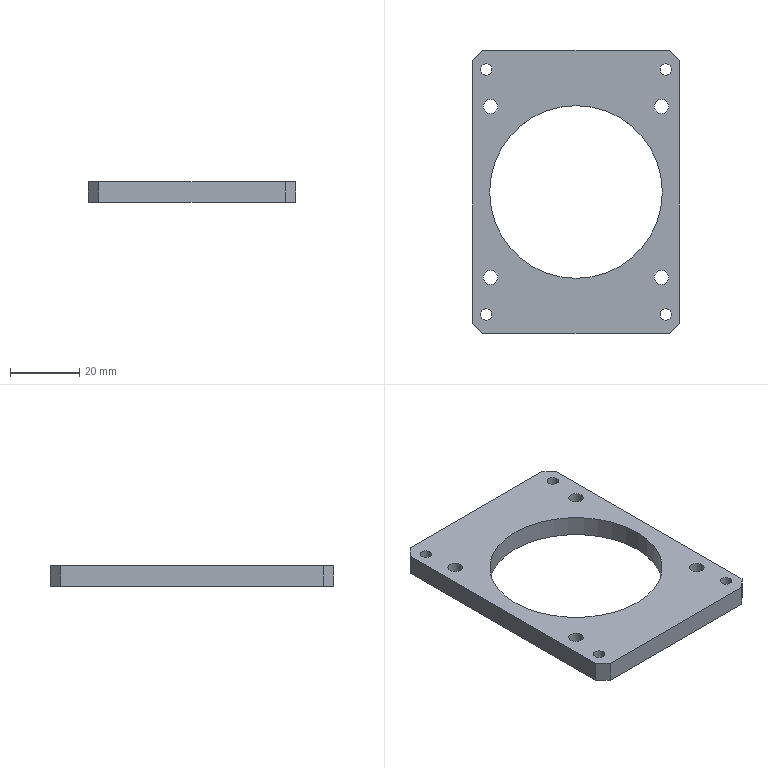Part | SolidWorks | features BaseBody 1 | 1 solid | 28 faces | box 60 x 82 x 6 mm | volume 17093 mm3 | cylinder 18 | plane 10 | commonest cylinder face diameters 3.3 x8 4.2 x8 50 x2
STEP:
#1=CARTESIAN_POINT('',(-24.35,35.5,6.));
#2=VERTEX_POINT('',#1);
#3=CARTESIAN_POINT('',(-27.65,35.5,6.));
#4=VERTEX_POINT('',#3);
#5=CARTESIAN_POINT('',(-26.,35.5,6.));
#6=DIRECTION('',(0.,0.,-1.));
#7=DIRECTION('',(-1.,0.,0.));
#8=AXIS2_PLACEMENT_3D('',#5,#6,#7);
#9=CIRCLE('',#8,1.65);
#10=EDGE_CURVE('',#2,#4,#9,.T.);
#11=ORIENTED_EDGE('',*,*,#10,.F.);
#12=CARTESIAN_POINT('',(-24.35,35.5,0.));
#13=VERTEX_POINT('',#12);
#14=CARTESIAN_POINT('',(-24.35,35.5,0.));
#15=DIRECTION('',(0.,0.,-1.));
#16=VECTOR('',#15,1000.);
#17=LINE('',#14,#16);
#18=EDGE_CURVE('',#2,#13,#17,.T.);
#19=ORIENTED_EDGE('',*,*,#18,.T.);
#20=CARTESIAN_POINT('',(-27.65,35.5,0.));
#21=VERTEX_POINT('',#20);
#22=CARTESIAN_POINT('',(-26.,35.5,0.));
#23=DIRECTION('',(0.,0.,1.));
#24=DIRECTION('',(-1.,0.,0.));
#25=AXIS2_PLACEMENT_3D('',#22,#23,#24);
#26=CIRCLE('',#25,1.65);
#27=EDGE_CURVE('',#21,#13,#26,.T.);
#28=ORIENTED_EDGE('',*,*,#27,.F.);
#29=CARTESIAN_POINT('',(-27.65,35.5,0.));
#30=DIRECTION('',(0.,0.,-1.));
#31=VECTOR('',#30,1000.);
#32=LINE('',#29,#31);
#33=EDGE_CURVE('',#4,#21,#32,.T.);
#34=ORIENTED_EDGE('',*,*,#33,.F.);
#35=EDGE_LOOP('',(#11,#19,#28,#34));
#36=FACE_OUTER_BOUND('',#35,.T.);
#37=CARTESIAN_POINT('',(-26.,35.5,0.));
#38=DIRECTION('',(0.,0.,-1.));
#39=DIRECTION('',(-1.,0.,0.));
#40=AXIS2_PLACEMENT_3D('',#37,#38,#39);
#41=CYLINDRICAL_SURFACE('',#40,1.65);
#42=ADVANCED_FACE('',(#36),#41,.F.);
#43=CARTESIAN_POINT('',(-24.35,-35.5,6.));
#44=VERTEX_POINT('',#43);
#45=CARTESIAN_POINT('',(-27.65,-35.5,6.));
#46=VERTEX_POINT('',#45);
#47=CARTESIAN_POINT('',(-26.,-35.5,6.));
#48=DIRECTION('',(0.,0.,-1.));
#49=DIRECTION('',(-1.,0.,0.));
#50=AXIS2_PLACEMENT_3D('',#47,#48,#49);
#51=CIRCLE('',#50,1.65);
#52=EDGE_CURVE('',#44,#46,#51,.T.);
#53=ORIENTED_EDGE('',*,*,#52,.F.);
#54=CARTESIAN_POINT('',(-24.35,-35.5,0.));
#55=VERTEX_POINT('',#54);
#56=CARTESIAN_POINT('',(-24.35,-35.5,0.));
#57=DIRECTION('',(0.,0.,-1.));
#58=VECTOR('',#57,1000.);
#59=LINE('',#56,#58);
#60=EDGE_CURVE('',#44,#55,#59,.T.);
#61=ORIENTED_EDGE('',*,*,#60,.T.);
#62=CARTESIAN_POINT('',(-27.65,-35.5,0.));
#63=VERTEX_POINT('',#62);
#64=CARTESIAN_POINT('',(-26.,-35.5,0.));
#65=DIRECTION('',(0.,0.,1.));
#66=DIRECTION('',(-1.,0.,0.));
#67=AXIS2_PLACEMENT_3D('',#64,#65,#66);
#68=CIRCLE('',#67,1.65);
#69=EDGE_CURVE('',#63,#55,#68,.T.);
#70=ORIENTED_EDGE('',*,*,#69,.F.);
#71=CARTESIAN_POINT('',(-27.65,-35.5,0.));
#72=DIRECTION('',(0.,0.,-1.));
#73=VECTOR('',#72,1000.);
#74=LINE('',#71,#73);
#75=EDGE_CURVE('',#46,#63,#74,.T.);
#76=ORIENTED_EDGE('',*,*,#75,.F.);
#77=EDGE_LOOP('',(#53,#61,#70,#76));
#78=FACE_OUTER_BOUND('',#77,.T.);
#79=CARTESIAN_POINT('',(-26.,-35.5,0.));
#80=DIRECTION('',(0.,0.,-1.));
#81=DIRECTION('',(-1.,0.,0.));
#82=AXIS2_PLACEMENT_3D('',#79,#80,#81);
#83=CYLINDRICAL_SURFACE('',#82,1.65);
#84=ADVANCED_FACE('',(#78),#83,.F.);
#85=CARTESIAN_POINT('',(27.65,35.5,6.));
#86=VERTEX_POINT('',#85);
#87=CARTESIAN_POINT('',(24.35,35.5,6.));
#88=VERTEX_POINT('',#87);
#89=CARTESIAN_POINT('',(26.,35.5,6.));
#90=DIRECTION('',(0.,0.,-1.));
#91=DIRECTION('',(-1.,0.,0.));
#92=AXIS2_PLACEMENT_3D('',#89,#90,#91);
#93=CIRCLE('',#92,1.65);
#94=EDGE_CURVE('',#86,#88,#93,.T.);
#95=ORIENTED_EDGE('',*,*,#94,.F.);
#96=CARTESIAN_POINT('',(27.65,35.5,0.));
#97=VERTEX_POINT('',#96);
#98=CARTESIAN_POINT('',(27.65,35.5,0.));
#99=DIRECTION('',(0.,0.,-1.));
#100=VECTOR('',#99,1000.);
#101=LINE('',#98,#100);
#102=EDGE_CURVE('',#86,#97,#101,.T.);
#103=ORIENTED_EDGE('',*,*,#102,.T.);
#104=CARTESIAN_POINT('',(24.35,35.5,0.));
#105=VERTEX_POINT('',#104);
#106=CARTESIAN_POINT('',(26.,35.5,0.));
#107=DIRECTION('',(0.,0.,1.));
#108=DIRECTION('',(-1.,0.,0.));
#109=AXIS2_PLACEMENT_3D('',#106,#107,#108);
#110=CIRCLE('',#109,1.65);
#111=EDGE_CURVE('',#105,#97,#110,.T.);
#112=ORIENTED_EDGE('',*,*,#111,.F.);
#113=CARTESIAN_POINT('',(24.35,35.5,0.));
#114=DIRECTION('',(0.,0.,-1.));
#115=VECTOR('',#114,1000.);
#116=LINE('',#113,#115);
#117=EDGE_CURVE('',#88,#105,#116,.T.);
#118=ORIENTED_EDGE('',*,*,#117,.F.);
#119=EDGE_LOOP('',(#95,#103,#112,#118));
#120=FACE_OUTER_BOUND('',#119,.T.);
#121=CARTESIAN_POINT('',(26.,35.5,0.));
#122=DIRECTION('',(0.,0.,-1.));
#123=DIRECTION('',(-1.,0.,0.));
#124=AXIS2_PLACEMENT_3D('',#121,#122,#123);
#125=CYLINDRICAL_SURFACE('',#124,1.65);
#126=ADVANCED_FACE('',(#120),#125,.F.);
#127=CARTESIAN_POINT('',(27.65,-35.5,6.));
#128=VERTEX_POINT('',#127);
#129=CARTESIAN_POINT('',(24.35,-35.5,6.));
#130=VERTEX_POINT('',#129);
#131=CARTESIAN_POINT('',(26.,-35.5,6.));
#132=DIRECTION('',(0.,0.,-1.));
#133=DIRECTION('',(-1.,0.,0.));
#134=AXIS2_PLACEMENT_3D('',#131,#132,#133);
#135=CIRCLE('',#134,1.65);
#136=EDGE_CURVE('',#128,#130,#135,.T.);
#137=ORIENTED_EDGE('',*,*,#136,.F.);
#138=CARTESIAN_POINT('',(27.65,-35.5,0.));
#139=VERTEX_POINT('',#138);
#140=CARTESIAN_POINT('',(27.65,-35.5,0.));
#141=DIRECTION('',(0.,0.,-1.));
#142=VECTOR('',#141,1000.);
#143=LINE('',#140,#142);
#144=EDGE_CURVE('',#128,#139,#143,.T.);
#145=ORIENTED_EDGE('',*,*,#144,.T.);
#146=CARTESIAN_POINT('',(24.35,-35.5,0.));
#147=VERTEX_POINT('',#146);
#148=CARTESIAN_POINT('',(26.,-35.5,0.));
#149=DIRECTION('',(0.,0.,1.));
#150=DIRECTION('',(-1.,0.,0.));
#151=AXIS2_PLACEMENT_3D('',#148,#149,#150);
#152=CIRCLE('',#151,1.65);
#153=EDGE_CURVE('',#147,#139,#152,.T.);
#154=ORIENTED_EDGE('',*,*,#153,.F.);
#155=CARTESIAN_POINT('',(24.35,-35.5,0.));
#156=DIRECTION('',(0.,0.,-1.));
#157=VECTOR('',#156,1000.);
#158=LINE('',#155,#157);
#159=EDGE_CURVE('',#130,#147,#158,.T.);
#160=ORIENTED_EDGE('',*,*,#159,.F.);
#161=EDGE_LOOP('',(#137,#145,#154,#160));
#162=FACE_OUTER_BOUND('',#161,.T.);
#163=CARTESIAN_POINT('',(26.,-35.5,0.));
#164=DIRECTION('',(0.,0.,-1.));
#165=DIRECTION('',(-1.,0.,0.));
#166=AXIS2_PLACEMENT_3D('',#163,#164,#165);
#167=CYLINDRICAL_SURFACE('',#166,1.65);
#168=ADVANCED_FACE('',(#162),#167,.F.);
#169=CARTESIAN_POINT('',(26.849,24.749,6.));
#170=VERTEX_POINT('',#169);
#171=CARTESIAN_POINT('',(22.649,24.749,6.));
#172=VERTEX_POINT('',#171);
#173=CARTESIAN_POINT('',(24.749,24.749,6.));
#174=DIRECTION('',(0.,0.,-1.));
#175=DIRECTION('',(-1.,0.,0.));
#176=AXIS2_PLACEMENT_3D('',#173,#174,#175);
#177=CIRCLE('',#176,2.1);
#178=EDGE_CURVE('',#170,#172,#177,.T.);
#179=ORIENTED_EDGE('',*,*,#178,.F.);
#180=CARTESIAN_POINT('',(26.849,24.749,0.));
#181=VERTEX_POINT('',#180);
#182=CARTESIAN_POINT('',(26.849,24.749,0.));
#183=DIRECTION('',(0.,0.,-1.));
#184=VECTOR('',#183,1000.);
#185=LINE('',#182,#184);
#186=EDGE_CURVE('',#170,#181,#185,.T.);
#187=ORIENTED_EDGE('',*,*,#186,.T.);
#188=CARTESIAN_POINT('',(22.649,24.749,0.));
#189=VERTEX_POINT('',#188);
#190=CARTESIAN_POINT('',(24.749,24.749,0.));
#191=DIRECTION('',(0.,0.,1.));
#192=DIRECTION('',(-1.,0.,0.));
#193=AXIS2_PLACEMENT_3D('',#190,#191,#192);
#194=CIRCLE('',#193,2.1);
#195=EDGE_CURVE('',#189,#181,#194,.T.);
#196=ORIENTED_EDGE('',*,*,#195,.F.);
#197=CARTESIAN_POINT('',(22.649,24.749,0.));
#198=DIRECTION('',(0.,0.,-1.));
#199=VECTOR('',#198,1000.);
#200=LINE('',#197,#199);
#201=EDGE_CURVE('',#172,#189,#200,.T.);
#202=ORIENTED_EDGE('',*,*,#201,.F.);
#203=EDGE_LOOP('',(#179,#187,#196,#202));
#204=FACE_OUTER_BOUND('',#203,.T.);
#205=CARTESIAN_POINT('',(24.749,24.749,0.));
#206=DIRECTION('',(0.,0.,-1.));
#207=DIRECTION('',(-1.,0.,0.));
#208=AXIS2_PLACEMENT_3D('',#205,#206,#207);
#209=CYLINDRICAL_SURFACE('',#208,2.1);
#210=ADVANCED_FACE('',(#204),#209,.F.);
#211=CARTESIAN_POINT('',(-22.649,24.749,6.));
#212=VERTEX_POINT('',#211);
#213=CARTESIAN_POINT('',(-26.849,24.749,6.));
#214=VERTEX_POINT('',#213);
#215=CARTESIAN_POINT('',(-24.749,24.749,6.));
#216=DIRECTION('',(0.,0.,-1.));
#217=DIRECTION('',(-1.,0.,0.));
#218=AXIS2_PLACEMENT_3D('',#215,#216,#217);
#219=CIRCLE('',#218,2.1);
#220=EDGE_CURVE('',#212,#214,#219,.T.);
#221=ORIENTED_EDGE('',*,*,#220,.F.);
#222=CARTESIAN_POINT('',(-22.649,24.749,0.));
#223=VERTEX_POINT('',#222);
#224=CARTESIAN_POINT('',(-22.649,24.749,0.));
#225=DIRECTION('',(0.,0.,-1.));
#226=VECTOR('',#225,1000.);
#227=LINE('',#224,#226);
#228=EDGE_CURVE('',#212,#223,#227,.T.);
#229=ORIENTED_EDGE('',*,*,#228,.T.);
#230=CARTESIAN_POINT('',(-26.849,24.749,0.));
#231=VERTEX_POINT('',#230);
#232=CARTESIAN_POINT('',(-24.749,24.749,0.));
#233=DIRECTION('',(0.,0.,1.));
#234=DIRECTION('',(-1.,0.,0.));
#235=AXIS2_PLACEMENT_3D('',#232,#233,#234);
#236=CIRCLE('',#235,2.1);
#237=EDGE_CURVE('',#231,#223,#236,.T.);
#238=ORIENTED_EDGE('',*,*,#237,.F.);
#239=CARTESIAN_POINT('',(-26.849,24.749,0.));
#240=DIRECTION('',(0.,0.,-1.));
#241=VECTOR('',#240,1000.);
#242=LINE('',#239,#241);
#243=EDGE_CURVE('',#214,#231,#242,.T.);
#244=ORIENTED_EDGE('',*,*,#243,.F.);
#245=EDGE_LOOP('',(#221,#229,#238,#244));
#246=FACE_OUTER_BOUND('',#245,.T.);
#247=CARTESIAN_POINT('',(-24.749,24.749,0.));
#248=DIRECTION('',(0.,0.,-1.));
#249=DIRECTION('',(-1.,0.,0.));
#250=AXIS2_PLACEMENT_3D('',#247,#248,#249);
#251=CYLINDRICAL_SURFACE('',#250,2.1);
#252=ADVANCED_FACE('',(#246),#251,.F.);
#253=CARTESIAN_POINT('',(-22.649,-24.749,6.));
#254=VERTEX_POINT('',#253);
#255=CARTESIAN_POINT('',(-26.849,-24.749,6.));
#256=VERTEX_POINT('',#255);
#257=CARTESIAN_POINT('',(-24.749,-24.749,6.));
#258=DIRECTION('',(0.,0.,-1.));
#259=DIRECTION('',(-1.,0.,0.));
#260=AXIS2_PLACEMENT_3D('',#257,#258,#259);
#261=CIRCLE('',#260,2.1);
#262=EDGE_CURVE('',#254,#256,#261,.T.);
#263=ORIENTED_EDGE('',*,*,#262,.F.);
#264=CARTESIAN_POINT('',(-22.649,-24.749,0.));
#265=VERTEX_POINT('',#264);
#266=CARTESIAN_POINT('',(-22.649,-24.749,0.));
#267=DIRECTION('',(0.,0.,-1.));
#268=VECTOR('',#267,1000.);
#269=LINE('',#266,#268);
#270=EDGE_CURVE('',#254,#265,#269,.T.);
#271=ORIENTED_EDGE('',*,*,#270,.T.);
#272=CARTESIAN_POINT('',(-26.849,-24.749,0.));
#273=VERTEX_POINT('',#272);
#274=CARTESIAN_POINT('',(-24.749,-24.749,0.));
#275=DIRECTION('',(0.,0.,1.));
#276=DIRECTION('',(-1.,0.,0.));
#277=AXIS2_PLACEMENT_3D('',#274,#275,#276);
#278=CIRCLE('',#277,2.1);
#279=EDGE_CURVE('',#273,#265,#278,.T.);
#280=ORIENTED_EDGE('',*,*,#279,.F.);
#281=CARTESIAN_POINT('',(-26.849,-24.749,0.));
#282=DIRECTION('',(0.,0.,-1.));
#283=VECTOR('',#282,1000.);
#284=LINE('',#281,#283);
#285=EDGE_CURVE('',#256,#273,#284,.T.);
#286=ORIENTED_EDGE('',*,*,#285,.F.);
#287=EDGE_LOOP('',(#263,#271,#280,#286));
#288=FACE_OUTER_BOUND('',#287,.T.);
#289=CARTESIAN_POINT('',(-24.749,-24.749,0.));
#290=DIRECTION('',(0.,0.,-1.));
#291=DIRECTION('',(-1.,0.,0.));
#292=AXIS2_PLACEMENT_3D('',#289,#290,#291);
#293=CYLINDRICAL_SURFACE('',#292,2.1);
#294=ADVANCED_FACE('',(#288),#293,.F.);
#295=CARTESIAN_POINT('',(26.849,-24.749,6.));
#296=VERTEX_POINT('',#295);
#297=CARTESIAN_POINT('',(22.649,-24.749,6.));
#298=VERTEX_POINT('',#297);
#299=CARTESIAN_POINT('',(24.749,-24.749,6.));
#300=DIRECTION('',(0.,0.,-1.));
#301=DIRECTION('',(-1.,0.,0.));
#302=AXIS2_PLACEMENT_3D('',#299,#300,#301);
#303=CIRCLE('',#302,2.1);
#304=EDGE_CURVE('',#296,#298,#303,.T.);
#305=ORIENTED_EDGE('',*,*,#304,.F.);
#306=CARTESIAN_POINT('',(26.849,-24.749,0.));
#307=VERTEX_POINT('',#306);
#308=CARTESIAN_POINT('',(26.849,-24.749,0.));
#309=DIRECTION('',(0.,0.,-1.));
#310=VECTOR('',#309,1000.);
#311=LINE('',#308,#310);
#312=EDGE_CURVE('',#296,#307,#311,.T.);
#313=ORIENTED_EDGE('',*,*,#312,.T.);
#314=CARTESIAN_POINT('',(22.649,-24.749,0.));
#315=VERTEX_POINT('',#314);
#316=CARTESIAN_POINT('',(24.749,-24.749,0.));
#317=DIRECTION('',(0.,0.,1.));
#318=DIRECTION('',(-1.,0.,0.));
#319=AXIS2_PLACEMENT_3D('',#316,#317,#318);
#320=CIRCLE('',#319,2.1);
#321=EDGE_CURVE('',#315,#307,#320,.T.);
#322=ORIENTED_EDGE('',*,*,#321,.F.);
#323=CARTESIAN_POINT('',(22.649,-24.749,0.));
#324=DIRECTION('',(0.,0.,-1.));
#325=VECTOR('',#324,1000.);
#326=LINE('',#323,#325);
#327=EDGE_CURVE('',#298,#315,#326,.T.);
#328=ORIENTED_EDGE('',*,*,#327,.F.);
#329=EDGE_LOOP('',(#305,#313,#322,#328));
#330=FACE_OUTER_BOUND('',#329,.T.);
#331=CARTESIAN_POINT('',(24.749,-24.749,0.));
#332=DIRECTION('',(0.,0.,-1.));
#333=DIRECTION('',(-1.,0.,0.));
#334=AXIS2_PLACEMENT_3D('',#331,#332,#333);
#335=CYLINDRICAL_SURFACE('',#334,2.1);
#336=ADVANCED_FACE('',(#330),#335,.F.);
#337=CARTESIAN_POINT('',(25.,0.,6.));
#338=VERTEX_POINT('',#337);
#339=CARTESIAN_POINT('',(-25.,0.,6.));
#340=VERTEX_POINT('',#339);
#341=CARTESIAN_POINT('',(0.,0.,6.));
#342=DIRECTION('',(0.,0.,-1.));
#343=DIRECTION('',(-1.,0.,0.));
#344=AXIS2_PLACEMENT_3D('',#341,#342,#343);
#345=CIRCLE('',#344,25.);
#346=EDGE_CURVE('',#338,#340,#345,.T.);
#347=ORIENTED_EDGE('',*,*,#346,.F.);
#348=CARTESIAN_POINT('',(25.,0.,0.));
#349=VERTEX_POINT('',#348);
#350=CARTESIAN_POINT('',(25.,0.,0.));
#351=DIRECTION('',(0.,0.,-1.));
#352=VECTOR('',#351,1000.);
#353=LINE('',#350,#352);
#354=EDGE_CURVE('',#338,#349,#353,.T.);
#355=ORIENTED_EDGE('',*,*,#354,.T.);
#356=CARTESIAN_POINT('',(-25.,0.,0.));
#357=VERTEX_POINT('',#356);
#358=CARTESIAN_POINT('',(0.,0.,0.));
#359=DIRECTION('',(0.,0.,1.));
#360=DIRECTION('',(-1.,0.,0.));
#361=AXIS2_PLACEMENT_3D('',#358,#359,#360);
#362=CIRCLE('',#361,25.);
#363=EDGE_CURVE('',#357,#349,#362,.T.);
#364=ORIENTED_EDGE('',*,*,#363,.F.);
#365=CARTESIAN_POINT('',(-25.,0.,0.));
#366=DIRECTION('',(0.,0.,-1.));
#367=VECTOR('',#366,1000.);
#368=LINE('',#365,#367);
#369=EDGE_CURVE('',#340,#357,#368,.T.);
#370=ORIENTED_EDGE('',*,*,#369,.F.);
#371=EDGE_LOOP('',(#347,#355,#364,#370));
#372=FACE_OUTER_BOUND('',#371,.T.);
#373=CARTESIAN_POINT('',(0.,0.,0.));
#374=DIRECTION('',(0.,0.,-1.));
#375=DIRECTION('',(-1.,0.,0.));
#376=AXIS2_PLACEMENT_3D('',#373,#374,#375);
#377=CYLINDRICAL_SURFACE('',#376,25.);
#378=ADVANCED_FACE('',(#372),#377,.F.);
#379=CARTESIAN_POINT('',(-26.,35.5,6.));
#380=DIRECTION('',(0.,0.,-1.));
#381=DIRECTION('',(-1.,0.,0.));
#382=AXIS2_PLACEMENT_3D('',#379,#380,#381);
#383=CIRCLE('',#382,1.65);
#384=EDGE_CURVE('',#4,#2,#383,.T.);
#385=ORIENTED_EDGE('',*,*,#384,.T.);
#386=ORIENTED_EDGE('',*,*,#10,.T.);
#387=EDGE_LOOP('',(#385,#386));
#388=FACE_BOUND('',#387,.T.);
#389=CARTESIAN_POINT('',(-26.,-35.5,6.));
#390=DIRECTION('',(0.,0.,-1.));
#391=DIRECTION('',(-1.,0.,0.));
#392=AXIS2_PLACEMENT_3D('',#389,#390,#391);
#393=CIRCLE('',#392,1.65);
#394=EDGE_CURVE('',#46,#44,#393,.T.);
#395=ORIENTED_EDGE('',*,*,#394,.T.);
#396=ORIENTED_EDGE('',*,*,#52,.T.);
#397=EDGE_LOOP('',(#395,#396));
#398=FACE_BOUND('',#397,.T.);
#399=CARTESIAN_POINT('',(26.,35.5,6.));
#400=DIRECTION('',(0.,0.,-1.));
#401=DIRECTION('',(-1.,0.,0.));
#402=AXIS2_PLACEMENT_3D('',#399,#400,#401);
#403=CIRCLE('',#402,1.65);
#404=EDGE_CURVE('',#88,#86,#403,.T.);
#405=ORIENTED_EDGE('',*,*,#404,.T.);
#406=ORIENTED_EDGE('',*,*,#94,.T.);
#407=EDGE_LOOP('',(#405,#406));
#408=FACE_BOUND('',#407,.T.);
#409=CARTESIAN_POINT('',(26.,-35.5,6.));
#410=DIRECTION('',(0.,0.,-1.));
#411=DIRECTION('',(-1.,0.,0.));
#412=AXIS2_PLACEMENT_3D('',#409,#410,#411);
#413=CIRCLE('',#412,1.65);
#414=EDGE_CURVE('',#130,#128,#413,.T.);
#415=ORIENTED_EDGE('',*,*,#414,.T.);
#416=ORIENTED_EDGE('',*,*,#136,.T.);
#417=EDGE_LOOP('',(#415,#416));
#418=FACE_BOUND('',#417,.T.);
#419=CARTESIAN_POINT('',(24.749,24.749,6.));
#420=DIRECTION('',(0.,0.,-1.));
#421=DIRECTION('',(-1.,0.,0.));
#422=AXIS2_PLACEMENT_3D('',#419,#420,#421);
#423=CIRCLE('',#422,2.1);
#424=EDGE_CURVE('',#172,#170,#423,.T.);
#425=ORIENTED_EDGE('',*,*,#424,.T.);
#426=ORIENTED_EDGE('',*,*,#178,.T.);
#427=EDGE_LOOP('',(#425,#426));
#428=FACE_BOUND('',#427,.T.);
#429=CARTESIAN_POINT('',(-24.749,24.749,6.));
#430=DIRECTION('',(0.,0.,-1.));
#431=DIRECTION('',(-1.,0.,0.));
#432=AXIS2_PLACEMENT_3D('',#429,#430,#431);
#433=CIRCLE('',#432,2.1);
#434=EDGE_CURVE('',#214,#212,#433,.T.);
#435=ORIENTED_EDGE('',*,*,#434,.T.);
#436=ORIENTED_EDGE('',*,*,#220,.T.);
#437=EDGE_LOOP('',(#435,#436));
#438=FACE_BOUND('',#437,.T.);
#439=CARTESIAN_POINT('',(-24.749,-24.749,6.));
#440=DIRECTION('',(0.,0.,-1.));
#441=DIRECTION('',(-1.,0.,0.));
#442=AXIS2_PLACEMENT_3D('',#439,#440,#441);
#443=CIRCLE('',#442,2.1);
#444=EDGE_CURVE('',#256,#254,#443,.T.);
#445=ORIENTED_EDGE('',*,*,#444,.T.);
#446=ORIENTED_EDGE('',*,*,#262,.T.);
#447=EDGE_LOOP('',(#445,#446));
#448=FACE_BOUND('',#447,.T.);
#449=CARTESIAN_POINT('',(24.749,-24.749,6.));
#450=DIRECTION('',(0.,0.,-1.));
#451=DIRECTION('',(-1.,0.,0.));
#452=AXIS2_PLACEMENT_3D('',#449,#450,#451);
#453=CIRCLE('',#452,2.1);
#454=EDGE_CURVE('',#298,#296,#453,.T.);
#455=ORIENTED_EDGE('',*,*,#454,.T.);
#456=ORIENTED_EDGE('',*,*,#304,.T.);
#457=EDGE_LOOP('',(#455,#456));
#458=FACE_BOUND('',#457,.T.);
#459=CARTESIAN_POINT('',(0.,0.,6.));
#460=DIRECTION('',(0.,0.,-1.));
#461=DIRECTION('',(-1.,0.,0.));
#462=AXIS2_PLACEMENT_3D('',#459,#460,#461);
#463=CIRCLE('',#462,25.);
#464=EDGE_CURVE('',#340,#338,#463,.T.);
#465=ORIENTED_EDGE('',*,*,#464,.T.);
#466=ORIENTED_EDGE('',*,*,#346,.T.);
#467=EDGE_LOOP('',(#465,#466));
#468=FACE_BOUND('',#467,.T.);
#469=CARTESIAN_POINT('',(30.,-38.,6.));
#470=VERTEX_POINT('',#469);
#471=CARTESIAN_POINT('',(30.,38.,6.));
#472=VERTEX_POINT('',#471);
#473=CARTESIAN_POINT('',(30.,0.,6.));
#474=DIRECTION('',(0.,1.,0.));
#475=VECTOR('',#474,1000.);
#476=LINE('',#473,#475);
#477=EDGE_CURVE('',#470,#472,#476,.T.);
#478=ORIENTED_EDGE('',*,*,#477,.T.);
#479=CARTESIAN_POINT('',(27.,41.,6.));
#480=VERTEX_POINT('',#479);
#481=CARTESIAN_POINT('',(30.,38.,6.));
#482=DIRECTION('',(-0.7071,0.7071,0.));
#483=VECTOR('',#482,1000.);
#484=LINE('',#481,#483);
#485=EDGE_CURVE('',#472,#480,#484,.T.);
#486=ORIENTED_EDGE('',*,*,#485,.T.);
#487=CARTESIAN_POINT('',(-27.,41.,6.));
#488=VERTEX_POINT('',#487);
#489=CARTESIAN_POINT('',(0.,41.,6.));
#490=DIRECTION('',(-1.,0.,0.));
#491=VECTOR('',#490,1000.);
#492=LINE('',#489,#491);
#493=EDGE_CURVE('',#480,#488,#492,.T.);
#494=ORIENTED_EDGE('',*,*,#493,.T.);
#495=CARTESIAN_POINT('',(-30.,38.,6.));
#496=VERTEX_POINT('',#495);
#497=CARTESIAN_POINT('',(-27.,41.,6.));
#498=DIRECTION('',(-0.7071,-0.7071,0.));
#499=VECTOR('',#498,1000.);
#500=LINE('',#497,#499);
#501=EDGE_CURVE('',#488,#496,#500,.T.);
#502=ORIENTED_EDGE('',*,*,#501,.T.);
#503=CARTESIAN_POINT('',(-30.,-38.,6.));
#504=VERTEX_POINT('',#503);
#505=CARTESIAN_POINT('',(-30.,0.,6.));
#506=DIRECTION('',(0.,-1.,0.));
#507=VECTOR('',#506,1000.);
#508=LINE('',#505,#507);
#509=EDGE_CURVE('',#496,#504,#508,.T.);
#510=ORIENTED_EDGE('',*,*,#509,.T.);
#511=CARTESIAN_POINT('',(-27.,-41.,6.));
#512=VERTEX_POINT('',#511);
#513=CARTESIAN_POINT('',(-30.,-38.,6.));
#514=DIRECTION('',(0.7071,-0.7071,0.));
#515=VECTOR('',#514,1000.);
#516=LINE('',#513,#515);
#517=EDGE_CURVE('',#504,#512,#516,.T.);
#518=ORIENTED_EDGE('',*,*,#517,.T.);
#519=CARTESIAN_POINT('',(27.,-41.,6.));
#520=VERTEX_POINT('',#519);
#521=CARTESIAN_POINT('',(0.,-41.,6.));
#522=DIRECTION('',(1.,0.,0.));
#523=VECTOR('',#522,1000.);
#524=LINE('',#521,#523);
#525=EDGE_CURVE('',#512,#520,#524,.T.);
#526=ORIENTED_EDGE('',*,*,#525,.T.);
#527=CARTESIAN_POINT('',(27.,-41.,6.));
#528=DIRECTION('',(0.7071,0.7071,0.));
#529=VECTOR('',#528,1000.);
#530=LINE('',#527,#529);
#531=EDGE_CURVE('',#520,#470,#530,.T.);
#532=ORIENTED_EDGE('',*,*,#531,.T.);
#533=EDGE_LOOP('',(#478,#486,#494,#502,#510,#518,#526,#532));
#534=FACE_OUTER_BOUND('',#533,.T.);
#535=CARTESIAN_POINT('',(0.,0.,6.));
#536=DIRECTION('',(0.,0.,1.));
#537=DIRECTION('',(1.,0.,0.));
#538=AXIS2_PLACEMENT_3D('',#535,#536,#537);
#539=PLANE('',#538);
#540=ADVANCED_FACE('',(#388,#398,#408,#418,#428,#438,#448,#458,#468,#534),#539,.T.);
#541=ORIENTED_EDGE('',*,*,#18,.F.);
#542=ORIENTED_EDGE('',*,*,#384,.F.);
#543=ORIENTED_EDGE('',*,*,#33,.T.);
#544=CARTESIAN_POINT('',(-26.,35.5,0.));
#545=DIRECTION('',(0.,0.,1.));
#546=DIRECTION('',(-1.,0.,0.));
#547=AXIS2_PLACEMENT_3D('',#544,#545,#546);
#548=CIRCLE('',#547,1.65);
#549=EDGE_CURVE('',#13,#21,#548,.T.);
#550=ORIENTED_EDGE('',*,*,#549,.F.);
#551=EDGE_LOOP('',(#541,#542,#543,#550));
#552=FACE_OUTER_BOUND('',#551,.T.);
#553=CARTESIAN_POINT('',(-26.,35.5,0.));
#554=DIRECTION('',(0.,0.,-1.));
#555=DIRECTION('',(-1.,0.,0.));
#556=AXIS2_PLACEMENT_3D('',#553,#554,#555);
#557=CYLINDRICAL_SURFACE('',#556,1.65);
#558=ADVANCED_FACE('',(#552),#557,.F.);
#559=ORIENTED_EDGE('',*,*,#60,.F.);
#560=ORIENTED_EDGE('',*,*,#394,.F.);
#561=ORIENTED_EDGE('',*,*,#75,.T.);
#562=CARTESIAN_POINT('',(-26.,-35.5,0.));
#563=DIRECTION('',(0.,0.,1.));
#564=DIRECTION('',(-1.,0.,0.));
#565=AXIS2_PLACEMENT_3D('',#562,#563,#564);
#566=CIRCLE('',#565,1.65);
#567=EDGE_CURVE('',#55,#63,#566,.T.);
#568=ORIENTED_EDGE('',*,*,#567,.F.);
#569=EDGE_LOOP('',(#559,#560,#561,#568));
#570=FACE_OUTER_BOUND('',#569,.T.);
#571=CARTESIAN_POINT('',(-26.,-35.5,0.));
#572=DIRECTION('',(0.,0.,-1.));
#573=DIRECTION('',(-1.,0.,0.));
#574=AXIS2_PLACEMENT_3D('',#571,#572,#573);
#575=CYLINDRICAL_SURFACE('',#574,1.65);
#576=ADVANCED_FACE('',(#570),#575,.F.);
#577=ORIENTED_EDGE('',*,*,#102,.F.);
#578=ORIENTED_EDGE('',*,*,#404,.F.);
#579=ORIENTED_EDGE('',*,*,#117,.T.);
#580=CARTESIAN_POINT('',(26.,35.5,0.));
#581=DIRECTION('',(0.,0.,1.));
#582=DIRECTION('',(-1.,0.,0.));
#583=AXIS2_PLACEMENT_3D('',#580,#581,#582);
#584=CIRCLE('',#583,1.65);
#585=EDGE_CURVE('',#97,#105,#584,.T.);
#586=ORIENTED_EDGE('',*,*,#585,.F.);
#587=EDGE_LOOP('',(#577,#578,#579,#586));
#588=FACE_OUTER_BOUND('',#587,.T.);
#589=CARTESIAN_POINT('',(26.,35.5,0.));
#590=DIRECTION('',(0.,0.,-1.));
#591=DIRECTION('',(-1.,0.,0.));
#592=AXIS2_PLACEMENT_3D('',#589,#590,#591);
#593=CYLINDRICAL_SURFACE('',#592,1.65);
#594=ADVANCED_FACE('',(#588),#593,.F.);
#595=ORIENTED_EDGE('',*,*,#144,.F.);
#596=ORIENTED_EDGE('',*,*,#414,.F.);
#597=ORIENTED_EDGE('',*,*,#159,.T.);
#598=CARTESIAN_POINT('',(26.,-35.5,0.));
#599=DIRECTION('',(0.,0.,1.));
#600=DIRECTION('',(-1.,0.,0.));
#601=AXIS2_PLACEMENT_3D('',#598,#599,#600);
#602=CIRCLE('',#601,1.65);
#603=EDGE_CURVE('',#139,#147,#602,.T.);
#604=ORIENTED_EDGE('',*,*,#603,.F.);
#605=EDGE_LOOP('',(#595,#596,#597,#604));
#606=FACE_OUTER_BOUND('',#605,.T.);
#607=CARTESIAN_POINT('',(26.,-35.5,0.));
#608=DIRECTION('',(0.,0.,-1.));
#609=DIRECTION('',(-1.,0.,0.));
#610=AXIS2_PLACEMENT_3D('',#607,#608,#609);
#611=CYLINDRICAL_SURFACE('',#610,1.65);
#612=ADVANCED_FACE('',(#606),#611,.F.);
#613=ORIENTED_EDGE('',*,*,#186,.F.);
#614=ORIENTED_EDGE('',*,*,#424,.F.);
#615=ORIENTED_EDGE('',*,*,#201,.T.);
#616=CARTESIAN_POINT('',(24.749,24.749,0.));
#617=DIRECTION('',(0.,0.,1.));
#618=DIRECTION('',(-1.,0.,0.));
#619=AXIS2_PLACEMENT_3D('',#616,#617,#618);
#620=CIRCLE('',#619,2.1);
#621=EDGE_CURVE('',#181,#189,#620,.T.);
#622=ORIENTED_EDGE('',*,*,#621,.F.);
#623=EDGE_LOOP('',(#613,#614,#615,#622));
#624=FACE_OUTER_BOUND('',#623,.T.);
#625=CARTESIAN_POINT('',(24.749,24.749,0.));
#626=DIRECTION('',(0.,0.,-1.));
#627=DIRECTION('',(-1.,0.,0.));
#628=AXIS2_PLACEMENT_3D('',#625,#626,#627);
#629=CYLINDRICAL_SURFACE('',#628,2.1);
#630=ADVANCED_FACE('',(#624),#629,.F.);
#631=ORIENTED_EDGE('',*,*,#228,.F.);
#632=ORIENTED_EDGE('',*,*,#434,.F.);
#633=ORIENTED_EDGE('',*,*,#243,.T.);
#634=CARTESIAN_POINT('',(-24.749,24.749,0.));
#635=DIRECTION('',(0.,0.,1.));
#636=DIRECTION('',(-1.,0.,0.));
#637=AXIS2_PLACEMENT_3D('',#634,#635,#636);
#638=CIRCLE('',#637,2.1);
#639=EDGE_CURVE('',#223,#231,#638,.T.);
#640=ORIENTED_EDGE('',*,*,#639,.F.);
#641=EDGE_LOOP('',(#631,#632,#633,#640));
#642=FACE_OUTER_BOUND('',#641,.T.);
#643=CARTESIAN_POINT('',(-24.749,24.749,0.));
#644=DIRECTION('',(0.,0.,-1.));
#645=DIRECTION('',(-1.,0.,0.));
#646=AXIS2_PLACEMENT_3D('',#643,#644,#645);
#647=CYLINDRICAL_SURFACE('',#646,2.1);
#648=ADVANCED_FACE('',(#642),#647,.F.);
#649=ORIENTED_EDGE('',*,*,#270,.F.);
#650=ORIENTED_EDGE('',*,*,#444,.F.);
#651=ORIENTED_EDGE('',*,*,#285,.T.);
#652=CARTESIAN_POINT('',(-24.749,-24.749,0.));
#653=DIRECTION('',(0.,0.,1.));
#654=DIRECTION('',(-1.,0.,0.));
#655=AXIS2_PLACEMENT_3D('',#652,#653,#654);
#656=CIRCLE('',#655,2.1);
#657=EDGE_CURVE('',#265,#273,#656,.T.);
#658=ORIENTED_EDGE('',*,*,#657,.F.);
#659=EDGE_LOOP('',(#649,#650,#651,#658));
#660=FACE_OUTER_BOUND('',#659,.T.);
#661=CARTESIAN_POINT('',(-24.749,-24.749,0.));
#662=DIRECTION('',(0.,0.,-1.));
#663=DIRECTION('',(-1.,0.,0.));
#664=AXIS2_PLACEMENT_3D('',#661,#662,#663);
#665=CYLINDRICAL_SURFACE('',#664,2.1);
#666=ADVANCED_FACE('',(#660),#665,.F.);
#667=ORIENTED_EDGE('',*,*,#312,.F.);
#668=ORIENTED_EDGE('',*,*,#454,.F.);
#669=ORIENTED_EDGE('',*,*,#327,.T.);
#670=CARTESIAN_POINT('',(24.749,-24.749,0.));
#671=DIRECTION('',(0.,0.,1.));
#672=DIRECTION('',(-1.,0.,0.));
#673=AXIS2_PLACEMENT_3D('',#670,#671,#672);
#674=CIRCLE('',#673,2.1);
#675=EDGE_CURVE('',#307,#315,#674,.T.);
#676=ORIENTED_EDGE('',*,*,#675,.F.);
#677=EDGE_LOOP('',(#667,#668,#669,#676));
#678=FACE_OUTER_BOUND('',#677,.T.);
#679=CARTESIAN_POINT('',(24.749,-24.749,0.));
#680=DIRECTION('',(0.,0.,-1.));
#681=DIRECTION('',(-1.,0.,0.));
#682=AXIS2_PLACEMENT_3D('',#679,#680,#681);
#683=CYLINDRICAL_SURFACE('',#682,2.1);
#684=ADVANCED_FACE('',(#678),#683,.F.);
#685=ORIENTED_EDGE('',*,*,#354,.F.);
#686=ORIENTED_EDGE('',*,*,#464,.F.);
#687=ORIENTED_EDGE('',*,*,#369,.T.);
#688=CARTESIAN_POINT('',(0.,0.,0.));
#689=DIRECTION('',(0.,0.,1.));
#690=DIRECTION('',(-1.,0.,0.));
#691=AXIS2_PLACEMENT_3D('',#688,#689,#690);
#692=CIRCLE('',#691,25.);
#693=EDGE_CURVE('',#349,#357,#692,.T.);
#694=ORIENTED_EDGE('',*,*,#693,.F.);
#695=EDGE_LOOP('',(#685,#686,#687,#694));
#696=FACE_OUTER_BOUND('',#695,.T.);
#697=CARTESIAN_POINT('',(0.,0.,0.));
#698=DIRECTION('',(0.,0.,-1.));
#699=DIRECTION('',(-1.,0.,0.));
#700=AXIS2_PLACEMENT_3D('',#697,#698,#699);
#701=CYLINDRICAL_SURFACE('',#700,25.);
#702=ADVANCED_FACE('',(#696),#701,.F.);
#703=CARTESIAN_POINT('',(30.,38.,0.));
#704=VERTEX_POINT('',#703);
#705=CARTESIAN_POINT('',(30.,38.,6.));
#706=DIRECTION('',(0.,0.,1.));
#707=VECTOR('',#706,1000.);
#708=LINE('',#705,#707);
#709=EDGE_CURVE('',#704,#472,#708,.T.);
#710=ORIENTED_EDGE('',*,*,#709,.F.);
#711=CARTESIAN_POINT('',(27.,41.,0.));
#712=VERTEX_POINT('',#711);
#713=CARTESIAN_POINT('',(27.,41.,0.));
#714=DIRECTION('',(0.7071,-0.7071,0.));
#715=VECTOR('',#714,1000.);
#716=LINE('',#713,#715);
#717=EDGE_CURVE('',#712,#704,#716,.T.);
#718=ORIENTED_EDGE('',*,*,#717,.F.);
#719=CARTESIAN_POINT('',(27.,41.,6.));
#720=DIRECTION('',(0.,0.,-1.));
#721=VECTOR('',#720,1000.);
#722=LINE('',#719,#721);
#723=EDGE_CURVE('',#480,#712,#722,.T.);
#724=ORIENTED_EDGE('',*,*,#723,.F.);
#725=ORIENTED_EDGE('',*,*,#485,.F.);
#726=EDGE_LOOP('',(#710,#718,#724,#725));
#727=FACE_OUTER_BOUND('',#726,.T.);
#728=CARTESIAN_POINT('',(27.,41.,6.));
#729=DIRECTION('',(-0.7071,-0.7071,0.));
#730=DIRECTION('',(0.7071,-0.7071,0.));
#731=AXIS2_PLACEMENT_3D('',#728,#729,#730);
#732=PLANE('',#731);
#733=ADVANCED_FACE('',(#727),#732,.F.);
#734=CARTESIAN_POINT('',(30.,-38.,0.));
#735=VERTEX_POINT('',#734);
#736=CARTESIAN_POINT('',(30.,-38.,6.));
#737=DIRECTION('',(0.,0.,1.));
#738=VECTOR('',#737,1000.);
#739=LINE('',#736,#738);
#740=EDGE_CURVE('',#735,#470,#739,.T.);
#741=ORIENTED_EDGE('',*,*,#740,.F.);
#742=CARTESIAN_POINT('',(30.,41.,0.));
#743=DIRECTION('',(0.,-1.,0.));
#744=VECTOR('',#743,1000.);
#745=LINE('',#742,#744);
#746=EDGE_CURVE('',#704,#735,#745,.T.);
#747=ORIENTED_EDGE('',*,*,#746,.F.);
#748=ORIENTED_EDGE('',*,*,#709,.T.);
#749=ORIENTED_EDGE('',*,*,#477,.F.);
#750=EDGE_LOOP('',(#741,#747,#748,#749));
#751=FACE_OUTER_BOUND('',#750,.T.);
#752=CARTESIAN_POINT('',(30.,41.,6.));
#753=DIRECTION('',(-1.,0.,0.));
#754=DIRECTION('',(0.,0.,1.));
#755=AXIS2_PLACEMENT_3D('',#752,#753,#754);
#756=PLANE('',#755);
#757=ADVANCED_FACE('',(#751),#756,.F.);
#758=CARTESIAN_POINT('',(27.,-41.,0.));
#759=VERTEX_POINT('',#758);
#760=CARTESIAN_POINT('',(27.,-41.,6.));
#761=DIRECTION('',(0.,0.,1.));
#762=VECTOR('',#761,1000.);
#763=LINE('',#760,#762);
#764=EDGE_CURVE('',#759,#520,#763,.T.);
#765=ORIENTED_EDGE('',*,*,#764,.F.);
#766=CARTESIAN_POINT('',(30.,-38.,0.));
#767=DIRECTION('',(-0.7071,-0.7071,0.));
#768=VECTOR('',#767,1000.);
#769=LINE('',#766,#768);
#770=EDGE_CURVE('',#735,#759,#769,.T.);
#771=ORIENTED_EDGE('',*,*,#770,.F.);
#772=ORIENTED_EDGE('',*,*,#740,.T.);
#773=ORIENTED_EDGE('',*,*,#531,.F.);
#774=EDGE_LOOP('',(#765,#771,#772,#773));
#775=FACE_OUTER_BOUND('',#774,.T.);
#776=CARTESIAN_POINT('',(30.,-38.,6.));
#777=DIRECTION('',(-0.7071,0.7071,0.));
#778=DIRECTION('',(-0.7071,-0.7071,0.));
#779=AXIS2_PLACEMENT_3D('',#776,#777,#778);
#780=PLANE('',#779);
#781=ADVANCED_FACE('',(#775),#780,.F.);
#782=CARTESIAN_POINT('',(-27.,-41.,0.));
#783=VERTEX_POINT('',#782);
#784=CARTESIAN_POINT('',(-27.,-41.,6.));
#785=DIRECTION('',(0.,0.,1.));
#786=VECTOR('',#785,1000.);
#787=LINE('',#784,#786);
#788=EDGE_CURVE('',#783,#512,#787,.T.);
#789=ORIENTED_EDGE('',*,*,#788,.F.);
#790=CARTESIAN_POINT('',(-30.,-41.,0.));
#791=DIRECTION('',(-1.,0.,0.));
#792=VECTOR('',#791,1000.);
#793=LINE('',#790,#792);
#794=EDGE_CURVE('',#759,#783,#793,.T.);
#795=ORIENTED_EDGE('',*,*,#794,.F.);
#796=ORIENTED_EDGE('',*,*,#764,.T.);
#797=ORIENTED_EDGE('',*,*,#525,.F.);
#798=EDGE_LOOP('',(#789,#795,#796,#797));
#799=FACE_OUTER_BOUND('',#798,.T.);
#800=CARTESIAN_POINT('',(-30.,-41.,6.));
#801=DIRECTION('',(0.,1.,0.));
#802=DIRECTION('',(0.,0.,1.));
#803=AXIS2_PLACEMENT_3D('',#800,#801,#802);
#804=PLANE('',#803);
#805=ADVANCED_FACE('',(#799),#804,.F.);
#806=CARTESIAN_POINT('',(-30.,-38.,0.));
#807=VERTEX_POINT('',#806);
#808=CARTESIAN_POINT('',(-30.,-38.,6.));
#809=DIRECTION('',(0.,0.,1.));
#810=VECTOR('',#809,1000.);
#811=LINE('',#808,#810);
#812=EDGE_CURVE('',#807,#504,#811,.T.);
#813=ORIENTED_EDGE('',*,*,#812,.F.);
#814=CARTESIAN_POINT('',(-27.,-41.,0.));
#815=DIRECTION('',(-0.7071,0.7071,0.));
#816=VECTOR('',#815,1000.);
#817=LINE('',#814,#816);
#818=EDGE_CURVE('',#783,#807,#817,.T.);
#819=ORIENTED_EDGE('',*,*,#818,.F.);
#820=ORIENTED_EDGE('',*,*,#788,.T.);
#821=ORIENTED_EDGE('',*,*,#517,.F.);
#822=EDGE_LOOP('',(#813,#819,#820,#821));
#823=FACE_OUTER_BOUND('',#822,.T.);
#824=CARTESIAN_POINT('',(-27.,-41.,6.));
#825=DIRECTION('',(0.7071,0.7071,0.));
#826=DIRECTION('',(-0.7071,0.7071,0.));
#827=AXIS2_PLACEMENT_3D('',#824,#825,#826);
#828=PLANE('',#827);
#829=ADVANCED_FACE('',(#823),#828,.F.);
#830=CARTESIAN_POINT('',(-30.,38.,0.));
#831=VERTEX_POINT('',#830);
#832=CARTESIAN_POINT('',(-30.,38.,6.));
#833=DIRECTION('',(0.,0.,1.));
#834=VECTOR('',#833,1000.);
#835=LINE('',#832,#834);
#836=EDGE_CURVE('',#831,#496,#835,.T.);
#837=ORIENTED_EDGE('',*,*,#836,.F.);
#838=CARTESIAN_POINT('',(-30.,41.,0.));
#839=DIRECTION('',(0.,1.,0.));
#840=VECTOR('',#839,1000.);
#841=LINE('',#838,#840);
#842=EDGE_CURVE('',#807,#831,#841,.T.);
#843=ORIENTED_EDGE('',*,*,#842,.F.);
#844=ORIENTED_EDGE('',*,*,#812,.T.);
#845=ORIENTED_EDGE('',*,*,#509,.F.);
#846=EDGE_LOOP('',(#837,#843,#844,#845));
#847=FACE_OUTER_BOUND('',#846,.T.);
#848=CARTESIAN_POINT('',(-30.,41.,6.));
#849=DIRECTION('',(1.,0.,0.));
#850=DIRECTION('',(0.,1.,0.));
#851=AXIS2_PLACEMENT_3D('',#848,#849,#850);
#852=PLANE('',#851);
#853=ADVANCED_FACE('',(#847),#852,.F.);
#854=CARTESIAN_POINT('',(-27.,41.,0.));
#855=VERTEX_POINT('',#854);
#856=CARTESIAN_POINT('',(-27.,41.,6.));
#857=DIRECTION('',(0.,0.,1.));
#858=VECTOR('',#857,1000.);
#859=LINE('',#856,#858);
#860=EDGE_CURVE('',#855,#488,#859,.T.);
#861=ORIENTED_EDGE('',*,*,#860,.F.);
#862=CARTESIAN_POINT('',(-30.,38.,0.));
#863=DIRECTION('',(0.7071,0.7071,0.));
#864=VECTOR('',#863,1000.);
#865=LINE('',#862,#864);
#866=EDGE_CURVE('',#831,#855,#865,.T.);
#867=ORIENTED_EDGE('',*,*,#866,.F.);
#868=ORIENTED_EDGE('',*,*,#836,.T.);
#869=ORIENTED_EDGE('',*,*,#501,.F.);
#870=EDGE_LOOP('',(#861,#867,#868,#869));
#871=FACE_OUTER_BOUND('',#870,.T.);
#872=CARTESIAN_POINT('',(-30.,38.,6.));
#873=DIRECTION('',(0.7071,-0.7071,0.));
#874=DIRECTION('',(0.7071,0.7071,0.));
#875=AXIS2_PLACEMENT_3D('',#872,#873,#874);
#876=PLANE('',#875);
#877=ADVANCED_FACE('',(#871),#876,.F.);
#878=ORIENTED_EDGE('',*,*,#860,.T.);
#879=ORIENTED_EDGE('',*,*,#493,.F.);
#880=ORIENTED_EDGE('',*,*,#723,.T.);
#881=CARTESIAN_POINT('',(-30.,41.,0.));
#882=DIRECTION('',(1.,0.,0.));
#883=VECTOR('',#882,1000.);
#884=LINE('',#881,#883);
#885=EDGE_CURVE('',#855,#712,#884,.T.);
#886=ORIENTED_EDGE('',*,*,#885,.F.);
#887=EDGE_LOOP('',(#878,#879,#880,#886));
#888=FACE_OUTER_BOUND('',#887,.T.);
#889=CARTESIAN_POINT('',(-30.,41.,6.));
#890=DIRECTION('',(0.,-1.,0.));
#891=DIRECTION('',(0.,0.,-1.));
#892=AXIS2_PLACEMENT_3D('',#889,#890,#891);
#893=PLANE('',#892);
#894=ADVANCED_FACE('',(#888),#893,.F.);
#895=ORIENTED_EDGE('',*,*,#69,.T.);
#896=ORIENTED_EDGE('',*,*,#567,.T.);
#897=EDGE_LOOP('',(#895,#896));
#898=FACE_BOUND('',#897,.T.);
#899=ORIENTED_EDGE('',*,*,#111,.T.);
#900=ORIENTED_EDGE('',*,*,#585,.T.);
#901=EDGE_LOOP('',(#899,#900));
#902=FACE_BOUND('',#901,.T.);
#903=ORIENTED_EDGE('',*,*,#153,.T.);
#904=ORIENTED_EDGE('',*,*,#603,.T.);
#905=EDGE_LOOP('',(#903,#904));
#906=FACE_BOUND('',#905,.T.);
#907=ORIENTED_EDGE('',*,*,#195,.T.);
#908=ORIENTED_EDGE('',*,*,#621,.T.);
#909=EDGE_LOOP('',(#907,#908));
#910=FACE_BOUND('',#909,.T.);
#911=ORIENTED_EDGE('',*,*,#237,.T.);
#912=ORIENTED_EDGE('',*,*,#639,.T.);
#913=EDGE_LOOP('',(#911,#912));
#914=FACE_BOUND('',#913,.T.);
#915=ORIENTED_EDGE('',*,*,#279,.T.);
#916=ORIENTED_EDGE('',*,*,#657,.T.);
#917=EDGE_LOOP('',(#915,#916));
#918=FACE_BOUND('',#917,.T.);
#919=ORIENTED_EDGE('',*,*,#321,.T.);
#920=ORIENTED_EDGE('',*,*,#675,.T.);
#921=EDGE_LOOP('',(#919,#920));
#922=FACE_BOUND('',#921,.T.);
#923=ORIENTED_EDGE('',*,*,#363,.T.);
#924=ORIENTED_EDGE('',*,*,#693,.T.);
#925=EDGE_LOOP('',(#923,#924));
#926=FACE_BOUND('',#925,.T.);
#927=ORIENTED_EDGE('',*,*,#866,.T.);
#928=ORIENTED_EDGE('',*,*,#885,.T.);
#929=ORIENTED_EDGE('',*,*,#717,.T.);
#930=ORIENTED_EDGE('',*,*,#746,.T.);
#931=ORIENTED_EDGE('',*,*,#770,.T.);
#932=ORIENTED_EDGE('',*,*,#794,.T.);
#933=ORIENTED_EDGE('',*,*,#818,.T.);
#934=ORIENTED_EDGE('',*,*,#842,.T.);
#935=EDGE_LOOP('',(#927,#928,#929,#930,#931,#932,#933,#934));
#936=FACE_OUTER_BOUND('',#935,.T.);
#937=ORIENTED_EDGE('',*,*,#27,.T.);
#938=ORIENTED_EDGE('',*,*,#549,.T.);
#939=EDGE_LOOP('',(#937,#938));
#940=FACE_BOUND('',#939,.T.);
#941=CARTESIAN_POINT('',(0.,0.,0.));
#942=DIRECTION('',(0.,0.,1.));
#943=DIRECTION('',(1.,0.,0.));
#944=AXIS2_PLACEMENT_3D('',#941,#942,#943);
#945=PLANE('',#944);
#946=ADVANCED_FACE('',(#898,#902,#906,#910,#914,#918,#922,#926,#936,#940),#945,.F.);
#947=CLOSED_SHELL('',(#42,#84,#126,#168,#210,#252,#294,#336,#378,#540,#558,#576,#594,#612,#630,#648,#666,#684,#702,#733,#757,#781,#805,#829,#853,#877,#894,#946));
#948=MANIFOLD_SOLID_BREP('',#947);
#949=CARTESIAN_POINT('',(0.,0.,0.));
#950=DIRECTION('',(0.,0.,1.));
#951=DIRECTION('',(1.,0.,0.));
#952=AXIS2_PLACEMENT_3D('',#949,#950,#951);
#953=(LENGTH_UNIT()NAMED_UNIT(*)SI_UNIT(.MILLI.,.METRE.));
#954=UNCERTAINTY_MEASURE_WITH_UNIT(LENGTH_MEASURE(0.00001),#953,'','');
#955=(NAMED_UNIT(*)PLANE_ANGLE_UNIT()SI_UNIT($,.RADIAN.));
#956=(NAMED_UNIT(*)SI_UNIT($,.STERADIAN.)SOLID_ANGLE_UNIT());
#957=(GEOMETRIC_REPRESENTATION_CONTEXT(3)GLOBAL_UNCERTAINTY_ASSIGNED_CONTEXT((#954))GLOBAL_UNIT_ASSIGNED_CONTEXT((#953,#955,#956))REPRESENTATION_CONTEXT('',''));
#958=ADVANCED_BREP_SHAPE_REPRESENTATION('',(#948,#952),#957);